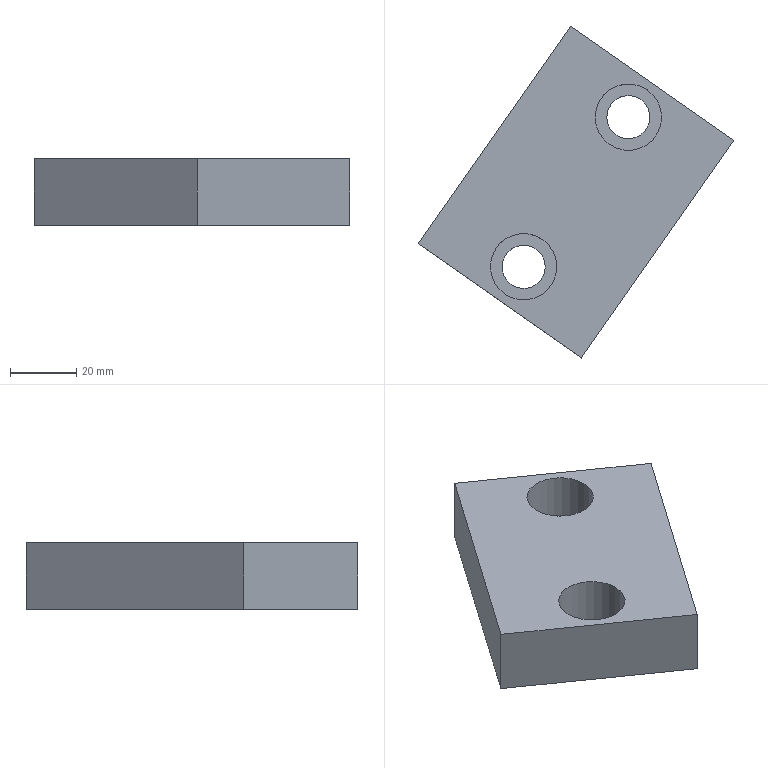Part | NX | features solid 2 | 1 solid | 12 faces | box 95.035 x 99.947 x 20 mm | volume 85611 mm3 | plane 8 | cylinder 4 | commonest cylinder face diameters 13 x2 20 x2
STEP:
#1=CARTESIAN_POINT('',(3.428,418.767,-110.));
#2=VERTEX_POINT('',#1);
#3=CARTESIAN_POINT('',(52.578,384.352,-110.));
#4=VERTEX_POINT('',#3);
#5=CARTESIAN_POINT('',(3.428,418.767,-110.));
#6=DIRECTION('',(0.8192,-0.5736,0.));
#7=VECTOR('',#6,1000.);
#8=LINE('',#5,#7);
#9=EDGE_CURVE('',#2,#4,#8,.T.);
#10=ORIENTED_EDGE('',*,*,#9,.T.);
#11=CARTESIAN_POINT('',(98.464,449.884,-110.));
#12=VERTEX_POINT('',#11);
#13=CARTESIAN_POINT('',(52.578,384.352,-110.));
#14=DIRECTION('',(0.5736,0.8192,0.));
#15=VECTOR('',#14,1000.);
#16=LINE('',#13,#15);
#17=EDGE_CURVE('',#4,#12,#16,.T.);
#18=ORIENTED_EDGE('',*,*,#17,.T.);
#19=CARTESIAN_POINT('',(49.315,484.299,-110.));
#20=VERTEX_POINT('',#19);
#21=CARTESIAN_POINT('',(98.464,449.884,-110.));
#22=DIRECTION('',(-0.8192,0.5736,0.));
#23=VECTOR('',#22,1000.);
#24=LINE('',#21,#23);
#25=EDGE_CURVE('',#12,#20,#24,.T.);
#26=ORIENTED_EDGE('',*,*,#25,.T.);
#27=CARTESIAN_POINT('',(49.315,484.299,-110.));
#28=DIRECTION('',(-0.5736,-0.8192,0.));
#29=VECTOR('',#28,1000.);
#30=LINE('',#27,#29);
#31=EDGE_CURVE('',#20,#2,#30,.T.);
#32=ORIENTED_EDGE('',*,*,#31,.T.);
#33=EDGE_LOOP('',(#10,#18,#26,#32));
#34=FACE_BOUND('',#33,.T.);
#35=CARTESIAN_POINT('',(60.984,448.661,-110.));
#36=VERTEX_POINT('',#35);
#37=CARTESIAN_POINT('',(66.719,456.852,-110.));
#38=DIRECTION('',(0.,0.,1.));
#39=DIRECTION('',(-0.5736,-0.8192,0.));
#40=AXIS2_PLACEMENT_3D('',#37,#38,#39);
#41=CIRCLE('',#40,10.);
#42=EDGE_CURVE('',#36,#36,#41,.T.);
#43=ORIENTED_EDGE('',*,*,#42,.F.);
#44=EDGE_LOOP('',(#43));
#45=FACE_BOUND('',#44,.T.);
#46=CARTESIAN_POINT('',(40.909,419.99,-110.));
#47=VERTEX_POINT('',#46);
#48=CARTESIAN_POINT('',(35.173,411.799,-110.));
#49=DIRECTION('',(0.,0.,-1.));
#50=DIRECTION('',(0.5736,0.8192,0.));
#51=AXIS2_PLACEMENT_3D('',#48,#49,#50);
#52=CIRCLE('',#51,10.);
#53=EDGE_CURVE('',#47,#47,#52,.T.);
#54=ORIENTED_EDGE('',*,*,#53,.T.);
#55=EDGE_LOOP('',(#54));
#56=FACE_BOUND('',#55,.T.);
#57=CARTESIAN_POINT('',(3.428,418.767,-110.));
#58=DIRECTION('',(0.,0.,1.));
#59=DIRECTION('',(0.5736,0.8192,0.));
#60=AXIS2_PLACEMENT_3D('',#57,#58,#59);
#61=PLANE('',#60);
#62=ADVANCED_FACE('',(#34,#45,#56),#61,.T.);
#63=CARTESIAN_POINT('',(38.901,417.123,-130.));
#64=VERTEX_POINT('',#63);
#65=CARTESIAN_POINT('',(35.173,411.799,-130.));
#66=DIRECTION('',(0.,0.,-1.));
#67=DIRECTION('',(0.5736,0.8192,0.));
#68=AXIS2_PLACEMENT_3D('',#65,#66,#67);
#69=CIRCLE('',#68,6.5);
#70=EDGE_CURVE('',#64,#64,#69,.T.);
#71=ORIENTED_EDGE('',*,*,#70,.T.);
#72=EDGE_LOOP('',(#71));
#73=FACE_BOUND('',#72,.T.);
#74=CARTESIAN_POINT('',(38.901,417.123,-124.));
#75=VERTEX_POINT('',#74);
#76=CARTESIAN_POINT('',(35.173,411.799,-124.));
#77=DIRECTION('',(0.,0.,-1.));
#78=DIRECTION('',(0.5736,0.8192,0.));
#79=AXIS2_PLACEMENT_3D('',#76,#77,#78);
#80=CIRCLE('',#79,6.5);
#81=EDGE_CURVE('',#75,#75,#80,.T.);
#82=ORIENTED_EDGE('',*,*,#81,.F.);
#83=EDGE_LOOP('',(#82));
#84=FACE_BOUND('',#83,.T.);
#85=CARTESIAN_POINT('',(35.173,411.799,-110.));
#86=DIRECTION('',(0.,0.,-1.));
#87=DIRECTION('',(-0.5736,-0.8192,0.));
#88=AXIS2_PLACEMENT_3D('',#85,#86,#87);
#89=CYLINDRICAL_SURFACE('',#88,6.5);
#90=ADVANCED_FACE('',(#73,#84),#89,.F.);
#91=CARTESIAN_POINT('',(3.428,418.767,-130.));
#92=VERTEX_POINT('',#91);
#93=CARTESIAN_POINT('',(52.578,384.352,-130.));
#94=VERTEX_POINT('',#93);
#95=CARTESIAN_POINT('',(3.428,418.767,-130.));
#96=DIRECTION('',(0.8192,-0.5736,0.));
#97=VECTOR('',#96,1000.);
#98=LINE('',#95,#97);
#99=EDGE_CURVE('',#92,#94,#98,.T.);
#100=ORIENTED_EDGE('',*,*,#99,.F.);
#101=CARTESIAN_POINT('',(49.315,484.299,-130.));
#102=VERTEX_POINT('',#101);
#103=CARTESIAN_POINT('',(49.315,484.299,-130.));
#104=DIRECTION('',(-0.5736,-0.8192,0.));
#105=VECTOR('',#104,1000.);
#106=LINE('',#103,#105);
#107=EDGE_CURVE('',#102,#92,#106,.T.);
#108=ORIENTED_EDGE('',*,*,#107,.F.);
#109=CARTESIAN_POINT('',(98.464,449.884,-130.));
#110=VERTEX_POINT('',#109);
#111=CARTESIAN_POINT('',(98.464,449.884,-130.));
#112=DIRECTION('',(-0.8192,0.5736,0.));
#113=VECTOR('',#112,1000.);
#114=LINE('',#111,#113);
#115=EDGE_CURVE('',#110,#102,#114,.T.);
#116=ORIENTED_EDGE('',*,*,#115,.F.);
#117=CARTESIAN_POINT('',(52.578,384.352,-130.));
#118=DIRECTION('',(0.5736,0.8192,0.));
#119=VECTOR('',#118,1000.);
#120=LINE('',#117,#119);
#121=EDGE_CURVE('',#94,#110,#120,.T.);
#122=ORIENTED_EDGE('',*,*,#121,.F.);
#123=EDGE_LOOP('',(#100,#108,#116,#122));
#124=FACE_BOUND('',#123,.T.);
#125=CARTESIAN_POINT('',(62.991,451.528,-130.));
#126=VERTEX_POINT('',#125);
#127=CARTESIAN_POINT('',(66.719,456.852,-130.));
#128=DIRECTION('',(0.,0.,1.));
#129=DIRECTION('',(-0.5736,-0.8192,0.));
#130=AXIS2_PLACEMENT_3D('',#127,#128,#129);
#131=CIRCLE('',#130,6.5);
#132=EDGE_CURVE('',#126,#126,#131,.T.);
#133=ORIENTED_EDGE('',*,*,#132,.T.);
#134=EDGE_LOOP('',(#133));
#135=FACE_BOUND('',#134,.T.);
#136=ORIENTED_EDGE('',*,*,#70,.F.);
#137=EDGE_LOOP('',(#136));
#138=FACE_BOUND('',#137,.T.);
#139=CARTESIAN_POINT('',(3.428,418.767,-130.));
#140=DIRECTION('',(0.,0.,1.));
#141=DIRECTION('',(0.5736,0.8192,0.));
#142=AXIS2_PLACEMENT_3D('',#139,#140,#141);
#143=PLANE('',#142);
#144=ADVANCED_FACE('',(#124,#135,#138),#143,.F.);
#145=ORIENTED_EDGE('',*,*,#99,.T.);
#146=CARTESIAN_POINT('',(52.578,384.352,-110.));
#147=DIRECTION('',(0.,0.,-1.));
#148=VECTOR('',#147,1000.);
#149=LINE('',#146,#148);
#150=EDGE_CURVE('',#4,#94,#149,.T.);
#151=ORIENTED_EDGE('',*,*,#150,.F.);
#152=ORIENTED_EDGE('',*,*,#9,.F.);
#153=CARTESIAN_POINT('',(3.428,418.767,-110.));
#154=DIRECTION('',(0.,0.,-1.));
#155=VECTOR('',#154,1000.);
#156=LINE('',#153,#155);
#157=EDGE_CURVE('',#2,#92,#156,.T.);
#158=ORIENTED_EDGE('',*,*,#157,.T.);
#159=EDGE_LOOP('',(#145,#151,#152,#158));
#160=FACE_BOUND('',#159,.T.);
#161=CARTESIAN_POINT('',(3.428,418.767,-110.));
#162=DIRECTION('',(-0.5736,-0.8192,0.));
#163=DIRECTION('',(-0.8192,0.5736,0.));
#164=AXIS2_PLACEMENT_3D('',#161,#162,#163);
#165=PLANE('',#164);
#166=ADVANCED_FACE('',(#160),#165,.T.);
#167=ORIENTED_EDGE('',*,*,#121,.T.);
#168=CARTESIAN_POINT('',(98.464,449.884,-110.));
#169=DIRECTION('',(0.,0.,-1.));
#170=VECTOR('',#169,1000.);
#171=LINE('',#168,#170);
#172=EDGE_CURVE('',#12,#110,#171,.T.);
#173=ORIENTED_EDGE('',*,*,#172,.F.);
#174=ORIENTED_EDGE('',*,*,#17,.F.);
#175=ORIENTED_EDGE('',*,*,#150,.T.);
#176=EDGE_LOOP('',(#167,#173,#174,#175));
#177=FACE_BOUND('',#176,.T.);
#178=CARTESIAN_POINT('',(52.578,384.352,-110.));
#179=DIRECTION('',(0.8192,-0.5736,0.));
#180=DIRECTION('',(-0.5736,-0.8192,0.));
#181=AXIS2_PLACEMENT_3D('',#178,#179,#180);
#182=PLANE('',#181);
#183=ADVANCED_FACE('',(#177),#182,.T.);
#184=ORIENTED_EDGE('',*,*,#115,.T.);
#185=CARTESIAN_POINT('',(49.315,484.299,-110.));
#186=DIRECTION('',(0.,0.,-1.));
#187=VECTOR('',#186,1000.);
#188=LINE('',#185,#187);
#189=EDGE_CURVE('',#20,#102,#188,.T.);
#190=ORIENTED_EDGE('',*,*,#189,.F.);
#191=ORIENTED_EDGE('',*,*,#25,.F.);
#192=ORIENTED_EDGE('',*,*,#172,.T.);
#193=EDGE_LOOP('',(#184,#190,#191,#192));
#194=FACE_BOUND('',#193,.T.);
#195=CARTESIAN_POINT('',(98.464,449.884,-110.));
#196=DIRECTION('',(0.5736,0.8192,0.));
#197=DIRECTION('',(0.8192,-0.5736,0.));
#198=AXIS2_PLACEMENT_3D('',#195,#196,#197);
#199=PLANE('',#198);
#200=ADVANCED_FACE('',(#194),#199,.T.);
#201=ORIENTED_EDGE('',*,*,#107,.T.);
#202=ORIENTED_EDGE('',*,*,#157,.F.);
#203=ORIENTED_EDGE('',*,*,#31,.F.);
#204=ORIENTED_EDGE('',*,*,#189,.T.);
#205=EDGE_LOOP('',(#201,#202,#203,#204));
#206=FACE_BOUND('',#205,.T.);
#207=CARTESIAN_POINT('',(49.315,484.299,-110.));
#208=DIRECTION('',(-0.8192,0.5736,0.));
#209=DIRECTION('',(0.5736,0.8192,0.));
#210=AXIS2_PLACEMENT_3D('',#207,#208,#209);
#211=PLANE('',#210);
#212=ADVANCED_FACE('',(#206),#211,.T.);
#213=CARTESIAN_POINT('',(62.991,451.528,-124.));
#214=VERTEX_POINT('',#213);
#215=CARTESIAN_POINT('',(66.719,456.852,-124.));
#216=DIRECTION('',(0.,0.,1.));
#217=DIRECTION('',(-0.5736,-0.8192,0.));
#218=AXIS2_PLACEMENT_3D('',#215,#216,#217);
#219=CIRCLE('',#218,6.5);
#220=EDGE_CURVE('',#214,#214,#219,.F.);
#221=ORIENTED_EDGE('',*,*,#220,.F.);
#222=EDGE_LOOP('',(#221));
#223=FACE_BOUND('',#222,.T.);
#224=ORIENTED_EDGE('',*,*,#132,.F.);
#225=EDGE_LOOP('',(#224));
#226=FACE_BOUND('',#225,.T.);
#227=CARTESIAN_POINT('',(66.719,456.852,-110.));
#228=DIRECTION('',(0.,0.,-1.));
#229=DIRECTION('',(-0.5736,-0.8192,0.));
#230=AXIS2_PLACEMENT_3D('',#227,#228,#229);
#231=CYLINDRICAL_SURFACE('',#230,6.5);
#232=ADVANCED_FACE('',(#223,#226),#231,.F.);
#233=CARTESIAN_POINT('',(60.984,448.661,-124.));
#234=VERTEX_POINT('',#233);
#235=CARTESIAN_POINT('',(66.719,456.852,-124.));
#236=DIRECTION('',(0.,0.,1.));
#237=DIRECTION('',(-0.5736,-0.8192,0.));
#238=AXIS2_PLACEMENT_3D('',#235,#236,#237);
#239=CIRCLE('',#238,10.);
#240=EDGE_CURVE('',#234,#234,#239,.T.);
#241=ORIENTED_EDGE('',*,*,#240,.T.);
#242=EDGE_LOOP('',(#241));
#243=FACE_BOUND('',#242,.T.);
#244=ORIENTED_EDGE('',*,*,#220,.T.);
#245=EDGE_LOOP('',(#244));
#246=FACE_BOUND('',#245,.T.);
#247=CARTESIAN_POINT('',(66.719,456.852,-124.));
#248=DIRECTION('',(0.,0.,-1.));
#249=DIRECTION('',(-0.5736,-0.8192,0.));
#250=AXIS2_PLACEMENT_3D('',#247,#248,#249);
#251=PLANE('',#250);
#252=ADVANCED_FACE('',(#243,#246),#251,.F.);
#253=ORIENTED_EDGE('',*,*,#42,.T.);
#254=EDGE_LOOP('',(#253));
#255=FACE_BOUND('',#254,.T.);
#256=ORIENTED_EDGE('',*,*,#240,.F.);
#257=EDGE_LOOP('',(#256));
#258=FACE_BOUND('',#257,.T.);
#259=CARTESIAN_POINT('',(66.719,456.852,-110.));
#260=DIRECTION('',(0.,0.,-1.));
#261=DIRECTION('',(-0.5736,-0.8192,0.));
#262=AXIS2_PLACEMENT_3D('',#259,#260,#261);
#263=CYLINDRICAL_SURFACE('',#262,10.);
#264=ADVANCED_FACE('',(#255,#258),#263,.F.);
#265=ORIENTED_EDGE('',*,*,#53,.F.);
#266=EDGE_LOOP('',(#265));
#267=FACE_BOUND('',#266,.T.);
#268=CARTESIAN_POINT('',(40.909,419.99,-124.));
#269=VERTEX_POINT('',#268);
#270=CARTESIAN_POINT('',(35.173,411.799,-124.));
#271=DIRECTION('',(0.,0.,-1.));
#272=DIRECTION('',(0.5736,0.8192,0.));
#273=AXIS2_PLACEMENT_3D('',#270,#271,#272);
#274=CIRCLE('',#273,10.);
#275=EDGE_CURVE('',#269,#269,#274,.T.);
#276=ORIENTED_EDGE('',*,*,#275,.T.);
#277=EDGE_LOOP('',(#276));
#278=FACE_BOUND('',#277,.T.);
#279=CARTESIAN_POINT('',(35.173,411.799,-110.));
#280=DIRECTION('',(0.,0.,-1.));
#281=DIRECTION('',(-0.5736,-0.8192,0.));
#282=AXIS2_PLACEMENT_3D('',#279,#280,#281);
#283=CYLINDRICAL_SURFACE('',#282,10.);
#284=ADVANCED_FACE('',(#267,#278),#283,.F.);
#285=ORIENTED_EDGE('',*,*,#81,.T.);
#286=EDGE_LOOP('',(#285));
#287=FACE_BOUND('',#286,.T.);
#288=ORIENTED_EDGE('',*,*,#275,.F.);
#289=EDGE_LOOP('',(#288));
#290=FACE_BOUND('',#289,.T.);
#291=CARTESIAN_POINT('',(35.173,411.799,-124.));
#292=DIRECTION('',(0.,0.,1.));
#293=DIRECTION('',(0.5736,0.8192,0.));
#294=AXIS2_PLACEMENT_3D('',#291,#292,#293);
#295=PLANE('',#294);
#296=ADVANCED_FACE('',(#287,#290),#295,.T.);
#297=CLOSED_SHELL('',(#62,#90,#144,#166,#183,#200,#212,#232,#252,#264,#284,#296));
#298=MANIFOLD_SOLID_BREP('',#297);
#299=(LENGTH_UNIT()NAMED_UNIT(*)SI_UNIT(.MILLI.,.METRE.));
#300=UNCERTAINTY_MEASURE_WITH_UNIT(LENGTH_MEASURE(0.00001),#299,'','');
#301=(NAMED_UNIT(*)PLANE_ANGLE_UNIT()SI_UNIT($,.RADIAN.));
#302=(NAMED_UNIT(*)SI_UNIT($,.STERADIAN.)SOLID_ANGLE_UNIT());
#303=(GEOMETRIC_REPRESENTATION_CONTEXT(3)GLOBAL_UNCERTAINTY_ASSIGNED_CONTEXT((#300))GLOBAL_UNIT_ASSIGNED_CONTEXT((#299,#301,#302))REPRESENTATION_CONTEXT('',''));
#304=ADVANCED_BREP_SHAPE_REPRESENTATION('',(#298),#303);